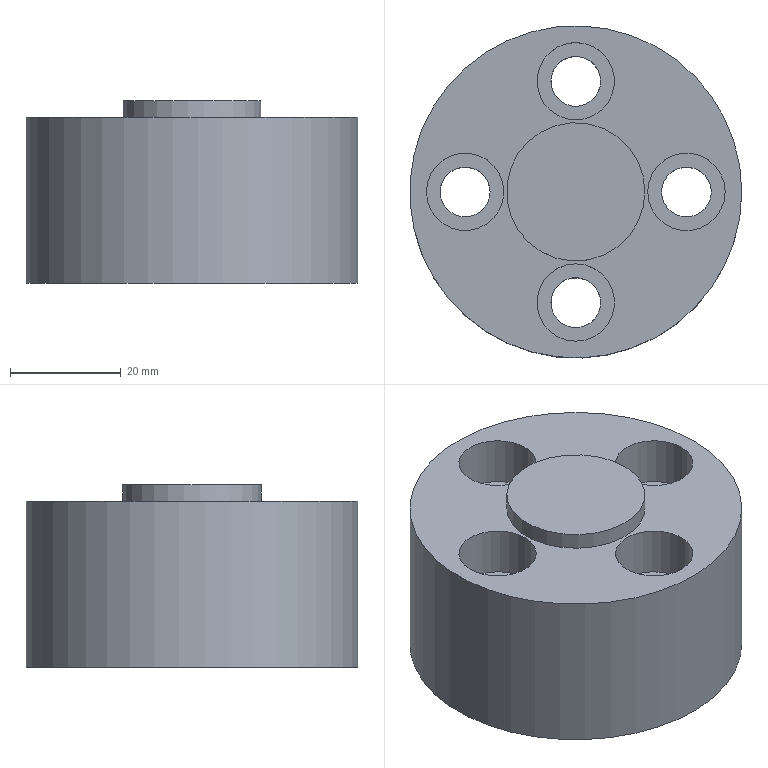NC program | NX | posted with a generic post | part box 60 x 60 x 33 mm
Whole program:
N10 G17 G21 G94 G90
(DRILLING , TOOL : ZXZ)
N12 T05 M6
N14 G54
N16 G17 G0 G90 X0. Y20. S3000 M3
N18 G43 Z30. H5
N20 G94 G81 G98 Z-4. F250. R0.
N22 X-20. Y0.
N24 X0. Y-20.
N26 X20. Y0.
N28 G80
N30 G0 X20. Y0. Z30.
N32 M5
(DRILLING_COPY , TOOL : 9.0ZT)
N34 T02 M6
N36 G54
N38 G17 G0 G90 X0. Y20. S1000 M3
N40 G43 Z30. H2
N42 G94 G73 G98 Z-36.204 F100. Q2. R0.
N44 X-20. Y0.
N46 X0. Y-20.
N48 X20. Y0.
N50 G80
N52 G0 X20. Y0. Z30.
N54 M5
N56 M2